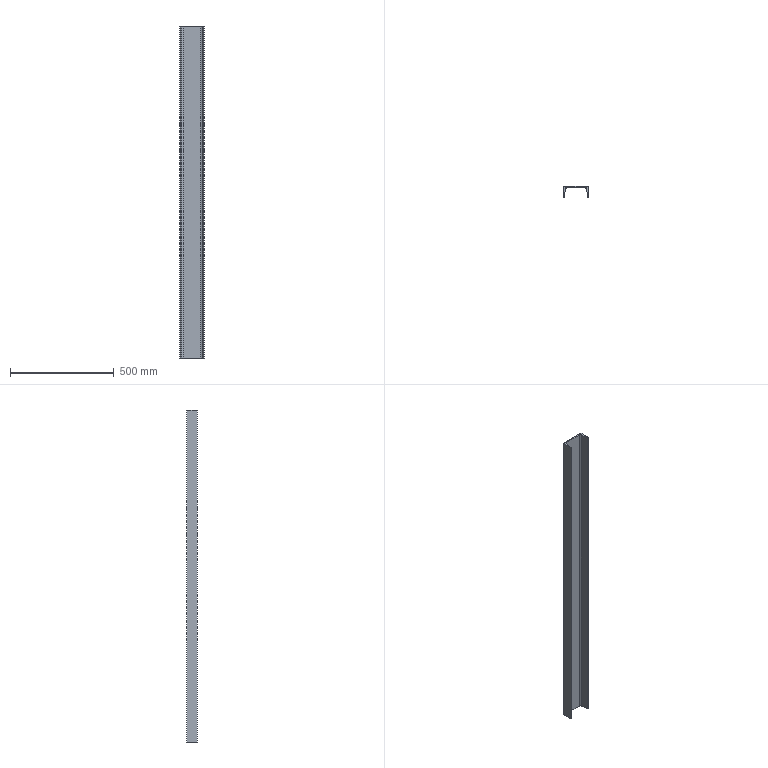Part | SolidWorks | features Extrusion 1 | 1 solid | 12 faces | box 120 x 53 x 1600 mm | volume 2068917 mm3 | plane 8 | cylinder 4 | commonest cylinder face diameters 9 x2 18 x2
STEP:
#1=CARTESIAN_POINT('',(-60.,0.,-800.));
#2=VERTEX_POINT('',#1);
#3=CARTESIAN_POINT('',(-60.,-53.,-800.));
#4=VERTEX_POINT('',#3);
#5=CARTESIAN_POINT('',(-60.,0.,-800.));
#6=DIRECTION('',(0.,-1.,0.));
#7=VECTOR('',#6,1000.);
#8=LINE('',#5,#7);
#9=EDGE_CURVE('',#2,#4,#8,.T.);
#10=ORIENTED_EDGE('',*,*,#9,.T.);
#11=CARTESIAN_POINT('',(-60.,-53.,800.));
#12=VERTEX_POINT('',#11);
#13=CARTESIAN_POINT('',(-60.,-53.,800.));
#14=DIRECTION('',(0.,0.,-1.));
#15=VECTOR('',#14,1000.);
#16=LINE('',#13,#15);
#17=EDGE_CURVE('',#12,#4,#16,.T.);
#18=ORIENTED_EDGE('',*,*,#17,.F.);
#19=CARTESIAN_POINT('',(-60.,0.,800.));
#20=VERTEX_POINT('',#19);
#21=CARTESIAN_POINT('',(-60.,0.,800.));
#22=DIRECTION('',(0.,-1.,0.));
#23=VECTOR('',#22,1000.);
#24=LINE('',#21,#23);
#25=EDGE_CURVE('',#20,#12,#24,.T.);
#26=ORIENTED_EDGE('',*,*,#25,.F.);
#27=CARTESIAN_POINT('',(-60.,0.,800.));
#28=DIRECTION('',(0.,0.,-1.));
#29=VECTOR('',#28,1000.);
#30=LINE('',#27,#29);
#31=EDGE_CURVE('',#20,#2,#30,.T.);
#32=ORIENTED_EDGE('',*,*,#31,.T.);
#33=EDGE_LOOP('',(#10,#18,#26,#32));
#34=FACE_OUTER_BOUND('',#33,.T.);
#35=CARTESIAN_POINT('',(-60.,0.,800.));
#36=DIRECTION('',(1.,0.,0.));
#37=DIRECTION('',(0.,0.,-1.));
#38=AXIS2_PLACEMENT_3D('',#35,#36,#37);
#39=PLANE('',#38);
#40=ADVANCED_FACE('',(#34),#39,.F.);
#41=CARTESIAN_POINT('',(-55.522,-48.948,-800.));
#42=VERTEX_POINT('',#41);
#43=CARTESIAN_POINT('',(-60.,-48.5,-800.));
#44=DIRECTION('',(0.,0.,1.));
#45=DIRECTION('',(1.,0.,0.));
#46=AXIS2_PLACEMENT_3D('',#43,#44,#45);
#47=CIRCLE('',#46,4.5);
#48=EDGE_CURVE('',#4,#42,#47,.T.);
#49=ORIENTED_EDGE('',*,*,#48,.T.);
#50=CARTESIAN_POINT('',(-55.522,-48.948,800.));
#51=VERTEX_POINT('',#50);
#52=CARTESIAN_POINT('',(-55.522,-48.948,800.));
#53=DIRECTION('',(0.,0.,-1.));
#54=VECTOR('',#53,1000.);
#55=LINE('',#52,#54);
#56=EDGE_CURVE('',#51,#42,#55,.T.);
#57=ORIENTED_EDGE('',*,*,#56,.F.);
#58=CARTESIAN_POINT('',(-60.,-48.5,800.));
#59=DIRECTION('',(0.,0.,1.));
#60=DIRECTION('',(1.,0.,0.));
#61=AXIS2_PLACEMENT_3D('',#58,#59,#60);
#62=CIRCLE('',#61,4.5);
#63=EDGE_CURVE('',#12,#51,#62,.T.);
#64=ORIENTED_EDGE('',*,*,#63,.F.);
#65=ORIENTED_EDGE('',*,*,#17,.T.);
#66=EDGE_LOOP('',(#49,#57,#64,#65));
#67=FACE_OUTER_BOUND('',#66,.T.);
#68=CARTESIAN_POINT('',(-60.,-48.5,800.));
#69=DIRECTION('',(0.,0.,-1.));
#70=DIRECTION('',(-1.,0.,0.));
#71=AXIS2_PLACEMENT_3D('',#68,#69,#70);
#72=CYLINDRICAL_SURFACE('',#71,4.5);
#73=ADVANCED_FACE('',(#67),#72,.T.);
#74=CARTESIAN_POINT('',(-51.988,-13.605,-800.));
#75=VERTEX_POINT('',#74);
#76=CARTESIAN_POINT('',(-55.522,-48.948,-800.));
#77=DIRECTION('',(0.09949,0.995,0.));
#78=VECTOR('',#77,1000.);
#79=LINE('',#76,#78);
#80=EDGE_CURVE('',#42,#75,#79,.T.);
#81=ORIENTED_EDGE('',*,*,#80,.T.);
#82=CARTESIAN_POINT('',(-51.988,-13.605,800.));
#83=VERTEX_POINT('',#82);
#84=CARTESIAN_POINT('',(-51.988,-13.605,800.));
#85=DIRECTION('',(0.,0.,-1.));
#86=VECTOR('',#85,1000.);
#87=LINE('',#84,#86);
#88=EDGE_CURVE('',#83,#75,#87,.T.);
#89=ORIENTED_EDGE('',*,*,#88,.F.);
#90=CARTESIAN_POINT('',(-55.522,-48.948,800.));
#91=DIRECTION('',(0.09949,0.995,0.));
#92=VECTOR('',#91,1000.);
#93=LINE('',#90,#92);
#94=EDGE_CURVE('',#51,#83,#93,.T.);
#95=ORIENTED_EDGE('',*,*,#94,.F.);
#96=ORIENTED_EDGE('',*,*,#56,.T.);
#97=EDGE_LOOP('',(#81,#89,#95,#96));
#98=FACE_OUTER_BOUND('',#97,.T.);
#99=CARTESIAN_POINT('',(-55.522,-48.948,800.));
#100=DIRECTION('',(-0.995,0.09949,0.));
#101=DIRECTION('',(-0.09949,-0.995,0.));
#102=AXIS2_PLACEMENT_3D('',#99,#100,#101);
#103=PLANE('',#102);
#104=ADVANCED_FACE('',(#98),#103,.F.);
#105=CARTESIAN_POINT('',(-43.033,-5.5,-800.));
#106=VERTEX_POINT('',#105);
#107=CARTESIAN_POINT('',(-43.033,-14.5,-800.));
#108=DIRECTION('',(0.,0.,-1.));
#109=DIRECTION('',(-1.,0.,0.));
#110=AXIS2_PLACEMENT_3D('',#107,#108,#109);
#111=CIRCLE('',#110,9.);
#112=EDGE_CURVE('',#75,#106,#111,.T.);
#113=ORIENTED_EDGE('',*,*,#112,.T.);
#114=CARTESIAN_POINT('',(-43.033,-5.5,800.));
#115=VERTEX_POINT('',#114);
#116=CARTESIAN_POINT('',(-43.033,-5.5,800.));
#117=DIRECTION('',(0.,0.,-1.));
#118=VECTOR('',#117,1000.);
#119=LINE('',#116,#118);
#120=EDGE_CURVE('',#115,#106,#119,.T.);
#121=ORIENTED_EDGE('',*,*,#120,.F.);
#122=CARTESIAN_POINT('',(-43.033,-14.5,800.));
#123=DIRECTION('',(0.,0.,-1.));
#124=DIRECTION('',(-1.,0.,0.));
#125=AXIS2_PLACEMENT_3D('',#122,#123,#124);
#126=CIRCLE('',#125,9.);
#127=EDGE_CURVE('',#83,#115,#126,.T.);
#128=ORIENTED_EDGE('',*,*,#127,.F.);
#129=ORIENTED_EDGE('',*,*,#88,.T.);
#130=EDGE_LOOP('',(#113,#121,#128,#129));
#131=FACE_OUTER_BOUND('',#130,.T.);
#132=CARTESIAN_POINT('',(-43.033,-14.5,800.));
#133=DIRECTION('',(0.,0.,-1.));
#134=DIRECTION('',(-1.,0.,0.));
#135=AXIS2_PLACEMENT_3D('',#132,#133,#134);
#136=CYLINDRICAL_SURFACE('',#135,9.);
#137=ADVANCED_FACE('',(#131),#136,.F.);
#138=CARTESIAN_POINT('',(43.033,-5.5,-800.));
#139=VERTEX_POINT('',#138);
#140=CARTESIAN_POINT('',(-43.033,-5.5,-800.));
#141=DIRECTION('',(1.,0.,0.));
#142=VECTOR('',#141,1000.);
#143=LINE('',#140,#142);
#144=EDGE_CURVE('',#106,#139,#143,.T.);
#145=ORIENTED_EDGE('',*,*,#144,.T.);
#146=CARTESIAN_POINT('',(43.033,-5.5,800.));
#147=VERTEX_POINT('',#146);
#148=CARTESIAN_POINT('',(43.033,-5.5,800.));
#149=DIRECTION('',(0.,0.,-1.));
#150=VECTOR('',#149,1000.);
#151=LINE('',#148,#150);
#152=EDGE_CURVE('',#147,#139,#151,.T.);
#153=ORIENTED_EDGE('',*,*,#152,.F.);
#154=CARTESIAN_POINT('',(-43.033,-5.5,800.));
#155=DIRECTION('',(1.,0.,0.));
#156=VECTOR('',#155,1000.);
#157=LINE('',#154,#156);
#158=EDGE_CURVE('',#115,#147,#157,.T.);
#159=ORIENTED_EDGE('',*,*,#158,.F.);
#160=ORIENTED_EDGE('',*,*,#120,.T.);
#161=EDGE_LOOP('',(#145,#153,#159,#160));
#162=FACE_OUTER_BOUND('',#161,.T.);
#163=CARTESIAN_POINT('',(-43.033,-5.5,800.));
#164=DIRECTION('',(0.,1.,0.));
#165=DIRECTION('',(-1.,0.,0.));
#166=AXIS2_PLACEMENT_3D('',#163,#164,#165);
#167=PLANE('',#166);
#168=ADVANCED_FACE('',(#162),#167,.F.);
#169=CARTESIAN_POINT('',(51.988,-13.605,-800.));
#170=VERTEX_POINT('',#169);
#171=CARTESIAN_POINT('',(43.033,-14.5,-800.));
#172=DIRECTION('',(0.,0.,-1.));
#173=DIRECTION('',(1.,0.,0.));
#174=AXIS2_PLACEMENT_3D('',#171,#172,#173);
#175=CIRCLE('',#174,9.);
#176=EDGE_CURVE('',#139,#170,#175,.T.);
#177=ORIENTED_EDGE('',*,*,#176,.T.);
#178=CARTESIAN_POINT('',(51.988,-13.605,800.));
#179=VERTEX_POINT('',#178);
#180=CARTESIAN_POINT('',(51.988,-13.605,800.));
#181=DIRECTION('',(0.,0.,-1.));
#182=VECTOR('',#181,1000.);
#183=LINE('',#180,#182);
#184=EDGE_CURVE('',#179,#170,#183,.T.);
#185=ORIENTED_EDGE('',*,*,#184,.F.);
#186=CARTESIAN_POINT('',(43.033,-14.5,800.));
#187=DIRECTION('',(0.,0.,-1.));
#188=DIRECTION('',(1.,0.,0.));
#189=AXIS2_PLACEMENT_3D('',#186,#187,#188);
#190=CIRCLE('',#189,9.);
#191=EDGE_CURVE('',#147,#179,#190,.T.);
#192=ORIENTED_EDGE('',*,*,#191,.F.);
#193=ORIENTED_EDGE('',*,*,#152,.T.);
#194=EDGE_LOOP('',(#177,#185,#192,#193));
#195=FACE_OUTER_BOUND('',#194,.T.);
#196=CARTESIAN_POINT('',(43.033,-14.5,800.));
#197=DIRECTION('',(0.,0.,-1.));
#198=DIRECTION('',(-1.,0.,0.));
#199=AXIS2_PLACEMENT_3D('',#196,#197,#198);
#200=CYLINDRICAL_SURFACE('',#199,9.);
#201=ADVANCED_FACE('',(#195),#200,.F.);
#202=CARTESIAN_POINT('',(55.522,-48.948,-800.));
#203=VERTEX_POINT('',#202);
#204=CARTESIAN_POINT('',(55.522,-48.948,-800.));
#205=DIRECTION('',(0.09949,-0.995,0.));
#206=VECTOR('',#205,1000.);
#207=LINE('',#204,#206);
#208=EDGE_CURVE('',#170,#203,#207,.T.);
#209=ORIENTED_EDGE('',*,*,#208,.T.);
#210=CARTESIAN_POINT('',(55.522,-48.948,800.));
#211=VERTEX_POINT('',#210);
#212=CARTESIAN_POINT('',(55.522,-48.948,800.));
#213=DIRECTION('',(0.,0.,-1.));
#214=VECTOR('',#213,1000.);
#215=LINE('',#212,#214);
#216=EDGE_CURVE('',#211,#203,#215,.T.);
#217=ORIENTED_EDGE('',*,*,#216,.F.);
#218=CARTESIAN_POINT('',(55.522,-48.948,800.));
#219=DIRECTION('',(0.09949,-0.995,0.));
#220=VECTOR('',#219,1000.);
#221=LINE('',#218,#220);
#222=EDGE_CURVE('',#179,#211,#221,.T.);
#223=ORIENTED_EDGE('',*,*,#222,.F.);
#224=ORIENTED_EDGE('',*,*,#184,.T.);
#225=EDGE_LOOP('',(#209,#217,#223,#224));
#226=FACE_OUTER_BOUND('',#225,.T.);
#227=CARTESIAN_POINT('',(55.522,-48.948,800.));
#228=DIRECTION('',(0.995,0.09949,0.));
#229=DIRECTION('',(-0.09949,0.995,0.));
#230=AXIS2_PLACEMENT_3D('',#227,#228,#229);
#231=PLANE('',#230);
#232=ADVANCED_FACE('',(#226),#231,.F.);
#233=CARTESIAN_POINT('',(60.,-53.,-800.));
#234=VERTEX_POINT('',#233);
#235=CARTESIAN_POINT('',(60.,-48.5,-800.));
#236=DIRECTION('',(0.,0.,1.));
#237=DIRECTION('',(-1.,0.,0.));
#238=AXIS2_PLACEMENT_3D('',#235,#236,#237);
#239=CIRCLE('',#238,4.5);
#240=EDGE_CURVE('',#203,#234,#239,.T.);
#241=ORIENTED_EDGE('',*,*,#240,.T.);
#242=CARTESIAN_POINT('',(60.,-53.,800.));
#243=VERTEX_POINT('',#242);
#244=CARTESIAN_POINT('',(60.,-53.,800.));
#245=DIRECTION('',(0.,0.,-1.));
#246=VECTOR('',#245,1000.);
#247=LINE('',#244,#246);
#248=EDGE_CURVE('',#243,#234,#247,.T.);
#249=ORIENTED_EDGE('',*,*,#248,.F.);
#250=CARTESIAN_POINT('',(60.,-48.5,800.));
#251=DIRECTION('',(0.,0.,1.));
#252=DIRECTION('',(-1.,0.,0.));
#253=AXIS2_PLACEMENT_3D('',#250,#251,#252);
#254=CIRCLE('',#253,4.5);
#255=EDGE_CURVE('',#211,#243,#254,.T.);
#256=ORIENTED_EDGE('',*,*,#255,.F.);
#257=ORIENTED_EDGE('',*,*,#216,.T.);
#258=EDGE_LOOP('',(#241,#249,#256,#257));
#259=FACE_OUTER_BOUND('',#258,.T.);
#260=CARTESIAN_POINT('',(60.,-48.5,800.));
#261=DIRECTION('',(0.,0.,-1.));
#262=DIRECTION('',(-1.,0.,0.));
#263=AXIS2_PLACEMENT_3D('',#260,#261,#262);
#264=CYLINDRICAL_SURFACE('',#263,4.5);
#265=ADVANCED_FACE('',(#259),#264,.T.);
#266=CARTESIAN_POINT('',(60.,0.,-800.));
#267=VERTEX_POINT('',#266);
#268=CARTESIAN_POINT('',(60.,0.,-800.));
#269=DIRECTION('',(0.,1.,0.));
#270=VECTOR('',#269,1000.);
#271=LINE('',#268,#270);
#272=EDGE_CURVE('',#234,#267,#271,.T.);
#273=ORIENTED_EDGE('',*,*,#272,.T.);
#274=CARTESIAN_POINT('',(60.,0.,800.));
#275=VERTEX_POINT('',#274);
#276=CARTESIAN_POINT('',(60.,0.,800.));
#277=DIRECTION('',(0.,0.,-1.));
#278=VECTOR('',#277,1000.);
#279=LINE('',#276,#278);
#280=EDGE_CURVE('',#275,#267,#279,.T.);
#281=ORIENTED_EDGE('',*,*,#280,.F.);
#282=CARTESIAN_POINT('',(60.,0.,800.));
#283=DIRECTION('',(0.,1.,0.));
#284=VECTOR('',#283,1000.);
#285=LINE('',#282,#284);
#286=EDGE_CURVE('',#243,#275,#285,.T.);
#287=ORIENTED_EDGE('',*,*,#286,.F.);
#288=ORIENTED_EDGE('',*,*,#248,.T.);
#289=EDGE_LOOP('',(#273,#281,#287,#288));
#290=FACE_OUTER_BOUND('',#289,.T.);
#291=CARTESIAN_POINT('',(60.,0.,800.));
#292=DIRECTION('',(-1.,0.,0.));
#293=DIRECTION('',(0.,-1.,0.));
#294=AXIS2_PLACEMENT_3D('',#291,#292,#293);
#295=PLANE('',#294);
#296=ADVANCED_FACE('',(#290),#295,.F.);
#297=CARTESIAN_POINT('',(60.,0.,-800.));
#298=DIRECTION('',(-1.,0.,0.));
#299=VECTOR('',#298,1000.);
#300=LINE('',#297,#299);
#301=EDGE_CURVE('',#267,#2,#300,.T.);
#302=ORIENTED_EDGE('',*,*,#301,.T.);
#303=ORIENTED_EDGE('',*,*,#31,.F.);
#304=CARTESIAN_POINT('',(60.,0.,800.));
#305=DIRECTION('',(-1.,0.,0.));
#306=VECTOR('',#305,1000.);
#307=LINE('',#304,#306);
#308=EDGE_CURVE('',#275,#20,#307,.T.);
#309=ORIENTED_EDGE('',*,*,#308,.F.);
#310=ORIENTED_EDGE('',*,*,#280,.T.);
#311=EDGE_LOOP('',(#302,#303,#309,#310));
#312=FACE_OUTER_BOUND('',#311,.T.);
#313=CARTESIAN_POINT('',(60.,0.,800.));
#314=DIRECTION('',(0.,-1.,0.));
#315=DIRECTION('',(1.,0.,0.));
#316=AXIS2_PLACEMENT_3D('',#313,#314,#315);
#317=PLANE('',#316);
#318=ADVANCED_FACE('',(#312),#317,.F.);
#319=ORIENTED_EDGE('',*,*,#25,.T.);
#320=ORIENTED_EDGE('',*,*,#63,.T.);
#321=ORIENTED_EDGE('',*,*,#94,.T.);
#322=ORIENTED_EDGE('',*,*,#127,.T.);
#323=ORIENTED_EDGE('',*,*,#158,.T.);
#324=ORIENTED_EDGE('',*,*,#191,.T.);
#325=ORIENTED_EDGE('',*,*,#222,.T.);
#326=ORIENTED_EDGE('',*,*,#255,.T.);
#327=ORIENTED_EDGE('',*,*,#286,.T.);
#328=ORIENTED_EDGE('',*,*,#308,.T.);
#329=EDGE_LOOP('',(#319,#320,#321,#322,#323,#324,#325,#326,#327,#328));
#330=FACE_OUTER_BOUND('',#329,.T.);
#331=CARTESIAN_POINT('',(-60.,-48.5,800.));
#332=DIRECTION('',(0.,0.,1.));
#333=DIRECTION('',(1.,0.,0.));
#334=AXIS2_PLACEMENT_3D('',#331,#332,#333);
#335=PLANE('',#334);
#336=ADVANCED_FACE('',(#330),#335,.T.);
#337=ORIENTED_EDGE('',*,*,#9,.F.);
#338=ORIENTED_EDGE('',*,*,#301,.F.);
#339=ORIENTED_EDGE('',*,*,#272,.F.);
#340=ORIENTED_EDGE('',*,*,#240,.F.);
#341=ORIENTED_EDGE('',*,*,#208,.F.);
#342=ORIENTED_EDGE('',*,*,#176,.F.);
#343=ORIENTED_EDGE('',*,*,#144,.F.);
#344=ORIENTED_EDGE('',*,*,#112,.F.);
#345=ORIENTED_EDGE('',*,*,#80,.F.);
#346=ORIENTED_EDGE('',*,*,#48,.F.);
#347=EDGE_LOOP('',(#337,#338,#339,#340,#341,#342,#343,#344,#345,#346));
#348=FACE_OUTER_BOUND('',#347,.T.);
#349=CARTESIAN_POINT('',(-60.,-48.5,-800.));
#350=DIRECTION('',(0.,0.,1.));
#351=DIRECTION('',(1.,0.,0.));
#352=AXIS2_PLACEMENT_3D('',#349,#350,#351);
#353=PLANE('',#352);
#354=ADVANCED_FACE('',(#348),#353,.F.);
#355=CLOSED_SHELL('',(#40,#73,#104,#137,#168,#201,#232,#265,#296,#318,#336,#354));
#356=MANIFOLD_SOLID_BREP('',#355);
#357=CARTESIAN_POINT('',(0.,0.,0.));
#358=DIRECTION('',(0.,0.,1.));
#359=DIRECTION('',(1.,0.,0.));
#360=AXIS2_PLACEMENT_3D('',#357,#358,#359);
#361=(LENGTH_UNIT()NAMED_UNIT(*)SI_UNIT(.MILLI.,.METRE.));
#362=UNCERTAINTY_MEASURE_WITH_UNIT(LENGTH_MEASURE(0.00001),#361,'','');
#363=(NAMED_UNIT(*)PLANE_ANGLE_UNIT()SI_UNIT($,.RADIAN.));
#364=(NAMED_UNIT(*)SI_UNIT($,.STERADIAN.)SOLID_ANGLE_UNIT());
#365=(GEOMETRIC_REPRESENTATION_CONTEXT(3)GLOBAL_UNCERTAINTY_ASSIGNED_CONTEXT((#362))GLOBAL_UNIT_ASSIGNED_CONTEXT((#361,#363,#364))REPRESENTATION_CONTEXT('',''));
#366=ADVANCED_BREP_SHAPE_REPRESENTATION('',(#356,#360),#365);